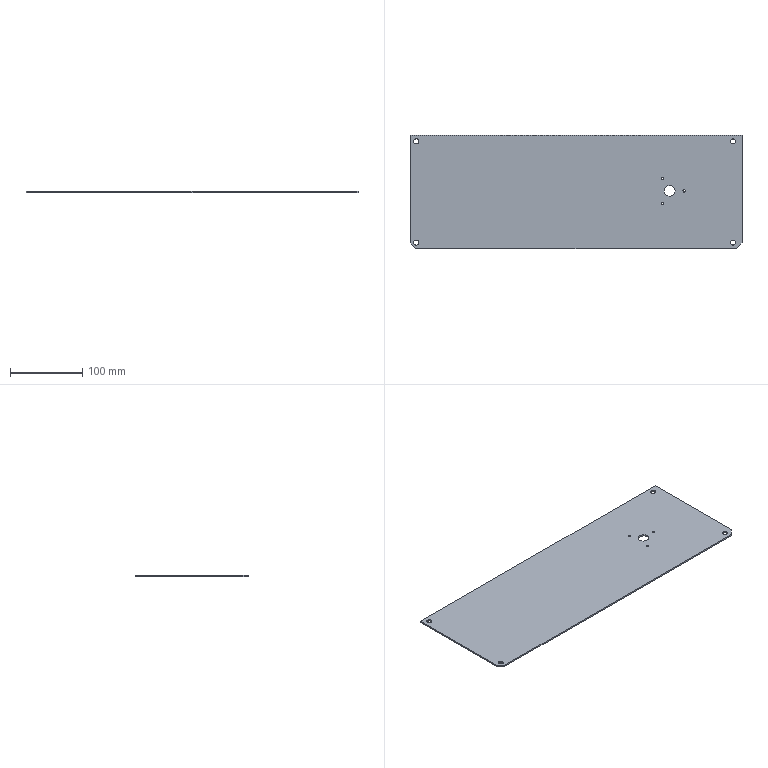Part | STEP file | Control Box Top Cover | 1 solid | 24 faces | box 459 x 157 x 2 mm | volume 143288 mm3 | cylinder 16 | plane 8 | commonest cylinder face diameters 7 x8 3.2 x6 15 x2
STEP:
#1=CARTESIAN_POINT('',(127.31,-1059.,2.));
#2=VERTEX_POINT('',#1);
#3=CARTESIAN_POINT('',(134.31,-1059.,2.));
#4=VERTEX_POINT('',#3);
#5=CARTESIAN_POINT('',(130.81,-1059.,2.));
#6=DIRECTION('',(0.,0.,1.));
#7=DIRECTION('',(-1.,0.,0.));
#8=AXIS2_PLACEMENT_3D('',#5,#6,#7);
#9=CIRCLE('',#8,3.5);
#10=EDGE_CURVE('',#2,#4,#9,.T.);
#11=ORIENTED_EDGE('',*,*,#10,.T.);
#12=CARTESIAN_POINT('',(134.31,-1059.,0.));
#13=VERTEX_POINT('',#12);
#14=CARTESIAN_POINT('',(134.31,-1059.,2.));
#15=DIRECTION('',(0.,0.,-1.));
#16=VECTOR('',#15,1000.);
#17=LINE('',#14,#16);
#18=EDGE_CURVE('',#4,#13,#17,.T.);
#19=ORIENTED_EDGE('',*,*,#18,.T.);
#20=CARTESIAN_POINT('',(127.31,-1059.,0.));
#21=VERTEX_POINT('',#20);
#22=CARTESIAN_POINT('',(130.81,-1059.,0.));
#23=DIRECTION('',(0.,0.,1.));
#24=DIRECTION('',(-1.,0.,0.));
#25=AXIS2_PLACEMENT_3D('',#22,#23,#24);
#26=CIRCLE('',#25,3.5);
#27=EDGE_CURVE('',#21,#13,#26,.T.);
#28=ORIENTED_EDGE('',*,*,#27,.F.);
#29=CARTESIAN_POINT('',(127.31,-1059.,2.));
#30=DIRECTION('',(0.,0.,-1.));
#31=VECTOR('',#30,1000.);
#32=LINE('',#29,#31);
#33=EDGE_CURVE('',#2,#21,#32,.T.);
#34=ORIENTED_EDGE('',*,*,#33,.F.);
#35=EDGE_LOOP('',(#11,#19,#28,#34));
#36=FACE_OUTER_BOUND('',#35,.T.);
#37=CARTESIAN_POINT('',(130.81,-1059.,2.));
#38=DIRECTION('',(0.,0.,-1.));
#39=DIRECTION('',(-1.,0.,0.));
#40=AXIS2_PLACEMENT_3D('',#37,#38,#39);
#41=CYLINDRICAL_SURFACE('',#40,3.5);
#42=ADVANCED_FACE('',(#36),#41,.F.);
#43=CARTESIAN_POINT('',(-310.69,-1199.,2.));
#44=VERTEX_POINT('',#43);
#45=CARTESIAN_POINT('',(-303.69,-1199.,2.));
#46=VERTEX_POINT('',#45);
#47=CARTESIAN_POINT('',(-307.19,-1199.,2.));
#48=DIRECTION('',(0.,0.,1.));
#49=DIRECTION('',(-1.,0.,0.));
#50=AXIS2_PLACEMENT_3D('',#47,#48,#49);
#51=CIRCLE('',#50,3.5);
#52=EDGE_CURVE('',#44,#46,#51,.T.);
#53=ORIENTED_EDGE('',*,*,#52,.T.);
#54=CARTESIAN_POINT('',(-303.69,-1199.,0.));
#55=VERTEX_POINT('',#54);
#56=CARTESIAN_POINT('',(-303.69,-1199.,2.));
#57=DIRECTION('',(0.,0.,-1.));
#58=VECTOR('',#57,1000.);
#59=LINE('',#56,#58);
#60=EDGE_CURVE('',#46,#55,#59,.T.);
#61=ORIENTED_EDGE('',*,*,#60,.T.);
#62=CARTESIAN_POINT('',(-310.69,-1199.,0.));
#63=VERTEX_POINT('',#62);
#64=CARTESIAN_POINT('',(-307.19,-1199.,0.));
#65=DIRECTION('',(0.,0.,1.));
#66=DIRECTION('',(-1.,0.,0.));
#67=AXIS2_PLACEMENT_3D('',#64,#65,#66);
#68=CIRCLE('',#67,3.5);
#69=EDGE_CURVE('',#63,#55,#68,.T.);
#70=ORIENTED_EDGE('',*,*,#69,.F.);
#71=CARTESIAN_POINT('',(-310.69,-1199.,2.));
#72=DIRECTION('',(0.,0.,-1.));
#73=VECTOR('',#72,1000.);
#74=LINE('',#71,#73);
#75=EDGE_CURVE('',#44,#63,#74,.T.);
#76=ORIENTED_EDGE('',*,*,#75,.F.);
#77=EDGE_LOOP('',(#53,#61,#70,#76));
#78=FACE_OUTER_BOUND('',#77,.T.);
#79=CARTESIAN_POINT('',(-307.19,-1199.,2.));
#80=DIRECTION('',(0.,0.,-1.));
#81=DIRECTION('',(-1.,0.,0.));
#82=AXIS2_PLACEMENT_3D('',#79,#80,#81);
#83=CYLINDRICAL_SURFACE('',#82,3.5);
#84=ADVANCED_FACE('',(#78),#83,.F.);
#85=CARTESIAN_POINT('',(-310.69,-1059.,2.));
#86=VERTEX_POINT('',#85);
#87=CARTESIAN_POINT('',(-303.69,-1059.,2.));
#88=VERTEX_POINT('',#87);
#89=CARTESIAN_POINT('',(-307.19,-1059.,2.));
#90=DIRECTION('',(0.,0.,1.));
#91=DIRECTION('',(-1.,0.,0.));
#92=AXIS2_PLACEMENT_3D('',#89,#90,#91);
#93=CIRCLE('',#92,3.5);
#94=EDGE_CURVE('',#86,#88,#93,.T.);
#95=ORIENTED_EDGE('',*,*,#94,.T.);
#96=CARTESIAN_POINT('',(-303.69,-1059.,0.));
#97=VERTEX_POINT('',#96);
#98=CARTESIAN_POINT('',(-303.69,-1059.,2.));
#99=DIRECTION('',(0.,0.,-1.));
#100=VECTOR('',#99,1000.);
#101=LINE('',#98,#100);
#102=EDGE_CURVE('',#88,#97,#101,.T.);
#103=ORIENTED_EDGE('',*,*,#102,.T.);
#104=CARTESIAN_POINT('',(-310.69,-1059.,0.));
#105=VERTEX_POINT('',#104);
#106=CARTESIAN_POINT('',(-307.19,-1059.,0.));
#107=DIRECTION('',(0.,0.,1.));
#108=DIRECTION('',(-1.,0.,0.));
#109=AXIS2_PLACEMENT_3D('',#106,#107,#108);
#110=CIRCLE('',#109,3.5);
#111=EDGE_CURVE('',#105,#97,#110,.T.);
#112=ORIENTED_EDGE('',*,*,#111,.F.);
#113=CARTESIAN_POINT('',(-310.69,-1059.,2.));
#114=DIRECTION('',(0.,0.,-1.));
#115=VECTOR('',#114,1000.);
#116=LINE('',#113,#115);
#117=EDGE_CURVE('',#86,#105,#116,.T.);
#118=ORIENTED_EDGE('',*,*,#117,.F.);
#119=EDGE_LOOP('',(#95,#103,#112,#118));
#120=FACE_OUTER_BOUND('',#119,.T.);
#121=CARTESIAN_POINT('',(-307.19,-1059.,2.));
#122=DIRECTION('',(0.,0.,-1.));
#123=DIRECTION('',(-1.,0.,0.));
#124=AXIS2_PLACEMENT_3D('',#121,#122,#123);
#125=CYLINDRICAL_SURFACE('',#124,3.5);
#126=ADVANCED_FACE('',(#120),#125,.F.);
#127=CARTESIAN_POINT('',(127.31,-1199.,2.));
#128=VERTEX_POINT('',#127);
#129=CARTESIAN_POINT('',(134.31,-1199.,2.));
#130=VERTEX_POINT('',#129);
#131=CARTESIAN_POINT('',(130.81,-1199.,2.));
#132=DIRECTION('',(0.,0.,1.));
#133=DIRECTION('',(-1.,0.,0.));
#134=AXIS2_PLACEMENT_3D('',#131,#132,#133);
#135=CIRCLE('',#134,3.5);
#136=EDGE_CURVE('',#128,#130,#135,.T.);
#137=ORIENTED_EDGE('',*,*,#136,.T.);
#138=CARTESIAN_POINT('',(134.31,-1199.,0.));
#139=VERTEX_POINT('',#138);
#140=CARTESIAN_POINT('',(134.31,-1199.,2.));
#141=DIRECTION('',(0.,0.,-1.));
#142=VECTOR('',#141,1000.);
#143=LINE('',#140,#142);
#144=EDGE_CURVE('',#130,#139,#143,.T.);
#145=ORIENTED_EDGE('',*,*,#144,.T.);
#146=CARTESIAN_POINT('',(127.31,-1199.,0.));
#147=VERTEX_POINT('',#146);
#148=CARTESIAN_POINT('',(130.81,-1199.,0.));
#149=DIRECTION('',(0.,0.,1.));
#150=DIRECTION('',(-1.,0.,0.));
#151=AXIS2_PLACEMENT_3D('',#148,#149,#150);
#152=CIRCLE('',#151,3.5);
#153=EDGE_CURVE('',#147,#139,#152,.T.);
#154=ORIENTED_EDGE('',*,*,#153,.F.);
#155=CARTESIAN_POINT('',(127.31,-1199.,2.));
#156=DIRECTION('',(0.,0.,-1.));
#157=VECTOR('',#156,1000.);
#158=LINE('',#155,#157);
#159=EDGE_CURVE('',#128,#147,#158,.T.);
#160=ORIENTED_EDGE('',*,*,#159,.F.);
#161=EDGE_LOOP('',(#137,#145,#154,#160));
#162=FACE_OUTER_BOUND('',#161,.T.);
#163=CARTESIAN_POINT('',(130.81,-1199.,2.));
#164=DIRECTION('',(0.,0.,-1.));
#165=DIRECTION('',(-1.,0.,0.));
#166=AXIS2_PLACEMENT_3D('',#163,#164,#165);
#167=CYLINDRICAL_SURFACE('',#166,3.5);
#168=ADVANCED_FACE('',(#162),#167,.F.);
#169=CARTESIAN_POINT('',(35.81,-1127.5,0.));
#170=VERTEX_POINT('',#169);
#171=CARTESIAN_POINT('',(50.81,-1127.5,0.));
#172=VERTEX_POINT('',#171);
#173=CARTESIAN_POINT('',(43.31,-1127.5,0.));
#174=DIRECTION('',(0.,0.,1.));
#175=DIRECTION('',(1.,0.,0.));
#176=AXIS2_PLACEMENT_3D('',#173,#174,#175);
#177=CIRCLE('',#176,7.5);
#178=EDGE_CURVE('',#170,#172,#177,.T.);
#179=ORIENTED_EDGE('',*,*,#178,.F.);
#180=CARTESIAN_POINT('',(35.81,-1127.5,2.));
#181=VERTEX_POINT('',#180);
#182=CARTESIAN_POINT('',(35.81,-1127.5,-8.));
#183=DIRECTION('',(0.,0.,1.));
#184=VECTOR('',#183,1000.);
#185=LINE('',#182,#184);
#186=EDGE_CURVE('',#170,#181,#185,.T.);
#187=ORIENTED_EDGE('',*,*,#186,.T.);
#188=CARTESIAN_POINT('',(50.81,-1127.5,2.));
#189=VERTEX_POINT('',#188);
#190=CARTESIAN_POINT('',(43.31,-1127.5,2.));
#191=DIRECTION('',(0.,0.,1.));
#192=DIRECTION('',(1.,0.,0.));
#193=AXIS2_PLACEMENT_3D('',#190,#191,#192);
#194=CIRCLE('',#193,7.5);
#195=EDGE_CURVE('',#181,#189,#194,.T.);
#196=ORIENTED_EDGE('',*,*,#195,.T.);
#197=CARTESIAN_POINT('',(50.81,-1127.5,-8.));
#198=DIRECTION('',(0.,0.,1.));
#199=VECTOR('',#198,1000.);
#200=LINE('',#197,#199);
#201=EDGE_CURVE('',#172,#189,#200,.T.);
#202=ORIENTED_EDGE('',*,*,#201,.F.);
#203=EDGE_LOOP('',(#179,#187,#196,#202));
#204=FACE_OUTER_BOUND('',#203,.T.);
#205=CARTESIAN_POINT('',(43.31,-1127.5,-8.));
#206=DIRECTION('',(0.,0.,1.));
#207=DIRECTION('',(1.,0.,0.));
#208=AXIS2_PLACEMENT_3D('',#205,#206,#207);
#209=CYLINDRICAL_SURFACE('',#208,7.5);
#210=ADVANCED_FACE('',(#204),#209,.F.);
#211=CARTESIAN_POINT('',(61.71,-1127.5,0.));
#212=VERTEX_POINT('',#211);
#213=CARTESIAN_POINT('',(64.91,-1127.5,0.));
#214=VERTEX_POINT('',#213);
#215=CARTESIAN_POINT('',(63.31,-1127.5,0.));
#216=DIRECTION('',(0.,0.,1.));
#217=DIRECTION('',(1.,0.,0.));
#218=AXIS2_PLACEMENT_3D('',#215,#216,#217);
#219=CIRCLE('',#218,1.6);
#220=EDGE_CURVE('',#212,#214,#219,.T.);
#221=ORIENTED_EDGE('',*,*,#220,.F.);
#222=CARTESIAN_POINT('',(61.71,-1127.5,2.));
#223=VERTEX_POINT('',#222);
#224=CARTESIAN_POINT('',(61.71,-1127.5,-8.));
#225=DIRECTION('',(0.,0.,1.));
#226=VECTOR('',#225,1000.);
#227=LINE('',#224,#226);
#228=EDGE_CURVE('',#212,#223,#227,.T.);
#229=ORIENTED_EDGE('',*,*,#228,.T.);
#230=CARTESIAN_POINT('',(64.91,-1127.5,2.));
#231=VERTEX_POINT('',#230);
#232=CARTESIAN_POINT('',(63.31,-1127.5,2.));
#233=DIRECTION('',(0.,0.,1.));
#234=DIRECTION('',(1.,0.,0.));
#235=AXIS2_PLACEMENT_3D('',#232,#233,#234);
#236=CIRCLE('',#235,1.6);
#237=EDGE_CURVE('',#223,#231,#236,.T.);
#238=ORIENTED_EDGE('',*,*,#237,.T.);
#239=CARTESIAN_POINT('',(64.91,-1127.5,-8.));
#240=DIRECTION('',(0.,0.,1.));
#241=VECTOR('',#240,1000.);
#242=LINE('',#239,#241);
#243=EDGE_CURVE('',#214,#231,#242,.T.);
#244=ORIENTED_EDGE('',*,*,#243,.F.);
#245=EDGE_LOOP('',(#221,#229,#238,#244));
#246=FACE_OUTER_BOUND('',#245,.T.);
#247=CARTESIAN_POINT('',(63.31,-1127.5,-8.));
#248=DIRECTION('',(0.,0.,1.));
#249=DIRECTION('',(1.,0.,0.));
#250=AXIS2_PLACEMENT_3D('',#247,#248,#249);
#251=CYLINDRICAL_SURFACE('',#250,1.6);
#252=ADVANCED_FACE('',(#246),#251,.F.);
#253=CARTESIAN_POINT('',(31.71,-1144.821,0.));
#254=VERTEX_POINT('',#253);
#255=CARTESIAN_POINT('',(34.91,-1144.821,0.));
#256=VERTEX_POINT('',#255);
#257=CARTESIAN_POINT('',(33.31,-1144.821,0.));
#258=DIRECTION('',(0.,0.,1.));
#259=DIRECTION('',(1.,0.,0.));
#260=AXIS2_PLACEMENT_3D('',#257,#258,#259);
#261=CIRCLE('',#260,1.6);
#262=EDGE_CURVE('',#254,#256,#261,.T.);
#263=ORIENTED_EDGE('',*,*,#262,.F.);
#264=CARTESIAN_POINT('',(31.71,-1144.821,2.));
#265=VERTEX_POINT('',#264);
#266=CARTESIAN_POINT('',(31.71,-1144.821,-8.));
#267=DIRECTION('',(0.,0.,1.));
#268=VECTOR('',#267,1000.);
#269=LINE('',#266,#268);
#270=EDGE_CURVE('',#254,#265,#269,.T.);
#271=ORIENTED_EDGE('',*,*,#270,.T.);
#272=CARTESIAN_POINT('',(34.91,-1144.821,2.));
#273=VERTEX_POINT('',#272);
#274=CARTESIAN_POINT('',(33.31,-1144.821,2.));
#275=DIRECTION('',(0.,0.,1.));
#276=DIRECTION('',(1.,0.,0.));
#277=AXIS2_PLACEMENT_3D('',#274,#275,#276);
#278=CIRCLE('',#277,1.6);
#279=EDGE_CURVE('',#265,#273,#278,.T.);
#280=ORIENTED_EDGE('',*,*,#279,.T.);
#281=CARTESIAN_POINT('',(34.91,-1144.821,-8.));
#282=DIRECTION('',(0.,0.,1.));
#283=VECTOR('',#282,1000.);
#284=LINE('',#281,#283);
#285=EDGE_CURVE('',#256,#273,#284,.T.);
#286=ORIENTED_EDGE('',*,*,#285,.F.);
#287=EDGE_LOOP('',(#263,#271,#280,#286));
#288=FACE_OUTER_BOUND('',#287,.T.);
#289=CARTESIAN_POINT('',(33.31,-1144.821,-8.));
#290=DIRECTION('',(0.,0.,1.));
#291=DIRECTION('',(1.,0.,0.));
#292=AXIS2_PLACEMENT_3D('',#289,#290,#291);
#293=CYLINDRICAL_SURFACE('',#292,1.6);
#294=ADVANCED_FACE('',(#288),#293,.F.);
#295=CARTESIAN_POINT('',(31.71,-1110.179,0.));
#296=VERTEX_POINT('',#295);
#297=CARTESIAN_POINT('',(34.91,-1110.179,0.));
#298=VERTEX_POINT('',#297);
#299=CARTESIAN_POINT('',(33.31,-1110.179,0.));
#300=DIRECTION('',(0.,0.,1.));
#301=DIRECTION('',(1.,0.,0.));
#302=AXIS2_PLACEMENT_3D('',#299,#300,#301);
#303=CIRCLE('',#302,1.6);
#304=EDGE_CURVE('',#296,#298,#303,.T.);
#305=ORIENTED_EDGE('',*,*,#304,.F.);
#306=CARTESIAN_POINT('',(31.71,-1110.179,2.));
#307=VERTEX_POINT('',#306);
#308=CARTESIAN_POINT('',(31.71,-1110.179,-8.));
#309=DIRECTION('',(0.,0.,1.));
#310=VECTOR('',#309,1000.);
#311=LINE('',#308,#310);
#312=EDGE_CURVE('',#296,#307,#311,.T.);
#313=ORIENTED_EDGE('',*,*,#312,.T.);
#314=CARTESIAN_POINT('',(34.91,-1110.179,2.));
#315=VERTEX_POINT('',#314);
#316=CARTESIAN_POINT('',(33.31,-1110.179,2.));
#317=DIRECTION('',(0.,0.,1.));
#318=DIRECTION('',(1.,0.,0.));
#319=AXIS2_PLACEMENT_3D('',#316,#317,#318);
#320=CIRCLE('',#319,1.6);
#321=EDGE_CURVE('',#307,#315,#320,.T.);
#322=ORIENTED_EDGE('',*,*,#321,.T.);
#323=CARTESIAN_POINT('',(34.91,-1110.179,-8.));
#324=DIRECTION('',(0.,0.,1.));
#325=VECTOR('',#324,1000.);
#326=LINE('',#323,#325);
#327=EDGE_CURVE('',#298,#315,#326,.T.);
#328=ORIENTED_EDGE('',*,*,#327,.F.);
#329=EDGE_LOOP('',(#305,#313,#322,#328));
#330=FACE_OUTER_BOUND('',#329,.T.);
#331=CARTESIAN_POINT('',(33.31,-1110.179,-8.));
#332=DIRECTION('',(0.,0.,1.));
#333=DIRECTION('',(1.,0.,0.));
#334=AXIS2_PLACEMENT_3D('',#331,#332,#333);
#335=CYLINDRICAL_SURFACE('',#334,1.6);
#336=ADVANCED_FACE('',(#330),#335,.F.);
#337=ORIENTED_EDGE('',*,*,#10,.F.);
#338=CARTESIAN_POINT('',(130.81,-1059.,2.));
#339=DIRECTION('',(0.,0.,1.));
#340=DIRECTION('',(-1.,0.,0.));
#341=AXIS2_PLACEMENT_3D('',#338,#339,#340);
#342=CIRCLE('',#341,3.5);
#343=EDGE_CURVE('',#4,#2,#342,.T.);
#344=ORIENTED_EDGE('',*,*,#343,.F.);
#345=EDGE_LOOP('',(#337,#344));
#346=FACE_BOUND('',#345,.T.);
#347=ORIENTED_EDGE('',*,*,#52,.F.);
#348=CARTESIAN_POINT('',(-307.19,-1199.,2.));
#349=DIRECTION('',(0.,0.,1.));
#350=DIRECTION('',(-1.,0.,0.));
#351=AXIS2_PLACEMENT_3D('',#348,#349,#350);
#352=CIRCLE('',#351,3.5);
#353=EDGE_CURVE('',#46,#44,#352,.T.);
#354=ORIENTED_EDGE('',*,*,#353,.F.);
#355=EDGE_LOOP('',(#347,#354));
#356=FACE_BOUND('',#355,.T.);
#357=CARTESIAN_POINT('',(143.31,-1199.5,2.));
#358=VERTEX_POINT('',#357);
#359=CARTESIAN_POINT('',(135.31,-1207.5,2.));
#360=VERTEX_POINT('',#359);
#361=CARTESIAN_POINT('',(143.31,-1199.5,2.));
#362=DIRECTION('',(-0.7071,-0.7071,0.));
#363=VECTOR('',#362,1000.);
#364=LINE('',#361,#363);
#365=EDGE_CURVE('',#358,#360,#364,.T.);
#366=ORIENTED_EDGE('',*,*,#365,.F.);
#367=CARTESIAN_POINT('',(143.31,-1050.5,2.));
#368=VERTEX_POINT('',#367);
#369=CARTESIAN_POINT('',(143.31,0.,2.));
#370=DIRECTION('',(0.,-1.,0.));
#371=VECTOR('',#370,1000.);
#372=LINE('',#369,#371);
#373=EDGE_CURVE('',#368,#358,#372,.T.);
#374=ORIENTED_EDGE('',*,*,#373,.F.);
#375=CARTESIAN_POINT('',(-315.69,-1050.5,2.));
#376=VERTEX_POINT('',#375);
#377=CARTESIAN_POINT('',(0.,-1050.5,2.));
#378=DIRECTION('',(1.,0.,0.));
#379=VECTOR('',#378,1000.);
#380=LINE('',#377,#379);
#381=EDGE_CURVE('',#376,#368,#380,.T.);
#382=ORIENTED_EDGE('',*,*,#381,.F.);
#383=CARTESIAN_POINT('',(-315.69,-1199.5,2.));
#384=VERTEX_POINT('',#383);
#385=CARTESIAN_POINT('',(-315.69,0.,2.));
#386=DIRECTION('',(0.,1.,0.));
#387=VECTOR('',#386,1000.);
#388=LINE('',#385,#387);
#389=EDGE_CURVE('',#384,#376,#388,.T.);
#390=ORIENTED_EDGE('',*,*,#389,.F.);
#391=CARTESIAN_POINT('',(-307.69,-1207.5,2.));
#392=VERTEX_POINT('',#391);
#393=CARTESIAN_POINT('',(-307.69,-1207.5,2.));
#394=DIRECTION('',(-0.7071,0.7071,0.));
#395=VECTOR('',#394,1000.);
#396=LINE('',#393,#395);
#397=EDGE_CURVE('',#392,#384,#396,.T.);
#398=ORIENTED_EDGE('',*,*,#397,.F.);
#399=CARTESIAN_POINT('',(0.,-1207.5,2.));
#400=DIRECTION('',(-1.,0.,0.));
#401=VECTOR('',#400,1000.);
#402=LINE('',#399,#401);
#403=EDGE_CURVE('',#360,#392,#402,.T.);
#404=ORIENTED_EDGE('',*,*,#403,.F.);
#405=EDGE_LOOP('',(#366,#374,#382,#390,#398,#404));
#406=FACE_OUTER_BOUND('',#405,.T.);
#407=ORIENTED_EDGE('',*,*,#94,.F.);
#408=CARTESIAN_POINT('',(-307.19,-1059.,2.));
#409=DIRECTION('',(0.,0.,1.));
#410=DIRECTION('',(-1.,0.,0.));
#411=AXIS2_PLACEMENT_3D('',#408,#409,#410);
#412=CIRCLE('',#411,3.5);
#413=EDGE_CURVE('',#88,#86,#412,.T.);
#414=ORIENTED_EDGE('',*,*,#413,.F.);
#415=EDGE_LOOP('',(#407,#414));
#416=FACE_BOUND('',#415,.T.);
#417=ORIENTED_EDGE('',*,*,#136,.F.);
#418=CARTESIAN_POINT('',(130.81,-1199.,2.));
#419=DIRECTION('',(0.,0.,1.));
#420=DIRECTION('',(-1.,0.,0.));
#421=AXIS2_PLACEMENT_3D('',#418,#419,#420);
#422=CIRCLE('',#421,3.5);
#423=EDGE_CURVE('',#130,#128,#422,.T.);
#424=ORIENTED_EDGE('',*,*,#423,.F.);
#425=EDGE_LOOP('',(#417,#424));
#426=FACE_BOUND('',#425,.T.);
#427=CARTESIAN_POINT('',(43.31,-1127.5,2.));
#428=DIRECTION('',(0.,0.,1.));
#429=DIRECTION('',(1.,0.,0.));
#430=AXIS2_PLACEMENT_3D('',#427,#428,#429);
#431=CIRCLE('',#430,7.5);
#432=EDGE_CURVE('',#189,#181,#431,.T.);
#433=ORIENTED_EDGE('',*,*,#432,.F.);
#434=ORIENTED_EDGE('',*,*,#195,.F.);
#435=EDGE_LOOP('',(#433,#434));
#436=FACE_BOUND('',#435,.T.);
#437=CARTESIAN_POINT('',(63.31,-1127.5,2.));
#438=DIRECTION('',(0.,0.,1.));
#439=DIRECTION('',(1.,0.,0.));
#440=AXIS2_PLACEMENT_3D('',#437,#438,#439);
#441=CIRCLE('',#440,1.6);
#442=EDGE_CURVE('',#231,#223,#441,.T.);
#443=ORIENTED_EDGE('',*,*,#442,.F.);
#444=ORIENTED_EDGE('',*,*,#237,.F.);
#445=EDGE_LOOP('',(#443,#444));
#446=FACE_BOUND('',#445,.T.);
#447=CARTESIAN_POINT('',(33.31,-1144.821,2.));
#448=DIRECTION('',(0.,0.,1.));
#449=DIRECTION('',(1.,0.,0.));
#450=AXIS2_PLACEMENT_3D('',#447,#448,#449);
#451=CIRCLE('',#450,1.6);
#452=EDGE_CURVE('',#273,#265,#451,.T.);
#453=ORIENTED_EDGE('',*,*,#452,.F.);
#454=ORIENTED_EDGE('',*,*,#279,.F.);
#455=EDGE_LOOP('',(#453,#454));
#456=FACE_BOUND('',#455,.T.);
#457=CARTESIAN_POINT('',(33.31,-1110.179,2.));
#458=DIRECTION('',(0.,0.,1.));
#459=DIRECTION('',(1.,0.,0.));
#460=AXIS2_PLACEMENT_3D('',#457,#458,#459);
#461=CIRCLE('',#460,1.6);
#462=EDGE_CURVE('',#315,#307,#461,.T.);
#463=ORIENTED_EDGE('',*,*,#462,.F.);
#464=ORIENTED_EDGE('',*,*,#321,.F.);
#465=EDGE_LOOP('',(#463,#464));
#466=FACE_BOUND('',#465,.T.);
#467=CARTESIAN_POINT('',(0.,0.,2.));
#468=DIRECTION('',(0.,0.,-1.));
#469=DIRECTION('',(-1.,0.,0.));
#470=AXIS2_PLACEMENT_3D('',#467,#468,#469);
#471=PLANE('',#470);
#472=ADVANCED_FACE('',(#346,#356,#406,#416,#426,#436,#446,#456,#466),#471,.F.);
#473=ORIENTED_EDGE('',*,*,#18,.F.);
#474=ORIENTED_EDGE('',*,*,#343,.T.);
#475=ORIENTED_EDGE('',*,*,#33,.T.);
#476=CARTESIAN_POINT('',(130.81,-1059.,0.));
#477=DIRECTION('',(0.,0.,1.));
#478=DIRECTION('',(-1.,0.,0.));
#479=AXIS2_PLACEMENT_3D('',#476,#477,#478);
#480=CIRCLE('',#479,3.5);
#481=EDGE_CURVE('',#13,#21,#480,.T.);
#482=ORIENTED_EDGE('',*,*,#481,.F.);
#483=EDGE_LOOP('',(#473,#474,#475,#482));
#484=FACE_OUTER_BOUND('',#483,.T.);
#485=CARTESIAN_POINT('',(130.81,-1059.,2.));
#486=DIRECTION('',(0.,0.,-1.));
#487=DIRECTION('',(-1.,0.,0.));
#488=AXIS2_PLACEMENT_3D('',#485,#486,#487);
#489=CYLINDRICAL_SURFACE('',#488,3.5);
#490=ADVANCED_FACE('',(#484),#489,.F.);
#491=ORIENTED_EDGE('',*,*,#60,.F.);
#492=ORIENTED_EDGE('',*,*,#353,.T.);
#493=ORIENTED_EDGE('',*,*,#75,.T.);
#494=CARTESIAN_POINT('',(-307.19,-1199.,0.));
#495=DIRECTION('',(0.,0.,1.));
#496=DIRECTION('',(-1.,0.,0.));
#497=AXIS2_PLACEMENT_3D('',#494,#495,#496);
#498=CIRCLE('',#497,3.5);
#499=EDGE_CURVE('',#55,#63,#498,.T.);
#500=ORIENTED_EDGE('',*,*,#499,.F.);
#501=EDGE_LOOP('',(#491,#492,#493,#500));
#502=FACE_OUTER_BOUND('',#501,.T.);
#503=CARTESIAN_POINT('',(-307.19,-1199.,2.));
#504=DIRECTION('',(0.,0.,-1.));
#505=DIRECTION('',(-1.,0.,0.));
#506=AXIS2_PLACEMENT_3D('',#503,#504,#505);
#507=CYLINDRICAL_SURFACE('',#506,3.5);
#508=ADVANCED_FACE('',(#502),#507,.F.);
#509=CARTESIAN_POINT('',(135.31,-1207.5,0.));
#510=VERTEX_POINT('',#509);
#511=CARTESIAN_POINT('',(135.31,-1207.5,2.));
#512=DIRECTION('',(0.,0.,-1.));
#513=VECTOR('',#512,1000.);
#514=LINE('',#511,#513);
#515=EDGE_CURVE('',#360,#510,#514,.T.);
#516=ORIENTED_EDGE('',*,*,#515,.F.);
#517=ORIENTED_EDGE('',*,*,#403,.T.);
#518=CARTESIAN_POINT('',(-307.69,-1207.5,0.));
#519=VERTEX_POINT('',#518);
#520=CARTESIAN_POINT('',(-307.69,-1207.5,2.));
#521=DIRECTION('',(0.,0.,1.));
#522=VECTOR('',#521,1000.);
#523=LINE('',#520,#522);
#524=EDGE_CURVE('',#519,#392,#523,.T.);
#525=ORIENTED_EDGE('',*,*,#524,.F.);
#526=CARTESIAN_POINT('',(-315.69,-1207.5,0.));
#527=DIRECTION('',(-1.,0.,0.));
#528=VECTOR('',#527,1000.);
#529=LINE('',#526,#528);
#530=EDGE_CURVE('',#510,#519,#529,.T.);
#531=ORIENTED_EDGE('',*,*,#530,.F.);
#532=EDGE_LOOP('',(#516,#517,#525,#531));
#533=FACE_OUTER_BOUND('',#532,.T.);
#534=CARTESIAN_POINT('',(-315.69,-1207.5,2.));
#535=DIRECTION('',(0.,1.,0.));
#536=DIRECTION('',(-1.,0.,0.));
#537=AXIS2_PLACEMENT_3D('',#534,#535,#536);
#538=PLANE('',#537);
#539=ADVANCED_FACE('',(#533),#538,.F.);
#540=ORIENTED_EDGE('',*,*,#515,.T.);
#541=CARTESIAN_POINT('',(143.31,-1199.5,0.));
#542=VERTEX_POINT('',#541);
#543=CARTESIAN_POINT('',(143.31,-1199.5,0.));
#544=DIRECTION('',(-0.7071,-0.7071,0.));
#545=VECTOR('',#544,1000.);
#546=LINE('',#543,#545);
#547=EDGE_CURVE('',#542,#510,#546,.T.);
#548=ORIENTED_EDGE('',*,*,#547,.F.);
#549=CARTESIAN_POINT('',(143.31,-1199.5,2.));
#550=DIRECTION('',(0.,0.,-1.));
#551=VECTOR('',#550,1000.);
#552=LINE('',#549,#551);
#553=EDGE_CURVE('',#358,#542,#552,.T.);
#554=ORIENTED_EDGE('',*,*,#553,.F.);
#555=ORIENTED_EDGE('',*,*,#365,.T.);
#556=EDGE_LOOP('',(#540,#548,#554,#555));
#557=FACE_OUTER_BOUND('',#556,.T.);
#558=CARTESIAN_POINT('',(143.31,-1199.5,2.));
#559=DIRECTION('',(-0.7071,0.7071,0.));
#560=DIRECTION('',(-0.7071,-0.7071,0.));
#561=AXIS2_PLACEMENT_3D('',#558,#559,#560);
#562=PLANE('',#561);
#563=ADVANCED_FACE('',(#557),#562,.F.);
#564=ORIENTED_EDGE('',*,*,#553,.T.);
#565=CARTESIAN_POINT('',(143.31,-1050.5,0.));
#566=VERTEX_POINT('',#565);
#567=CARTESIAN_POINT('',(143.31,-1050.5,0.));
#568=DIRECTION('',(0.,-1.,0.));
#569=VECTOR('',#568,1000.);
#570=LINE('',#567,#569);
#571=EDGE_CURVE('',#566,#542,#570,.T.);
#572=ORIENTED_EDGE('',*,*,#571,.F.);
#573=CARTESIAN_POINT('',(143.31,-1050.5,2.));
#574=DIRECTION('',(0.,0.,-1.));
#575=VECTOR('',#574,1000.);
#576=LINE('',#573,#575);
#577=EDGE_CURVE('',#368,#566,#576,.T.);
#578=ORIENTED_EDGE('',*,*,#577,.F.);
#579=ORIENTED_EDGE('',*,*,#373,.T.);
#580=EDGE_LOOP('',(#564,#572,#578,#579));
#581=FACE_OUTER_BOUND('',#580,.T.);
#582=CARTESIAN_POINT('',(143.31,-1050.5,2.));
#583=DIRECTION('',(-1.,0.,0.));
#584=DIRECTION('',(0.,0.,1.));
#585=AXIS2_PLACEMENT_3D('',#582,#583,#584);
#586=PLANE('',#585);
#587=ADVANCED_FACE('',(#581),#586,.F.);
#588=CARTESIAN_POINT('',(-315.69,-1050.5,0.));
#589=VERTEX_POINT('',#588);
#590=CARTESIAN_POINT('',(-315.69,-1050.5,2.));
#591=DIRECTION('',(0.,0.,-1.));
#592=VECTOR('',#591,1000.);
#593=LINE('',#590,#592);
#594=EDGE_CURVE('',#376,#589,#593,.T.);
#595=ORIENTED_EDGE('',*,*,#594,.F.);
#596=ORIENTED_EDGE('',*,*,#381,.T.);
#597=ORIENTED_EDGE('',*,*,#577,.T.);
#598=CARTESIAN_POINT('',(-315.69,-1050.5,0.));
#599=DIRECTION('',(1.,0.,0.));
#600=VECTOR('',#599,1000.);
#601=LINE('',#598,#600);
#602=EDGE_CURVE('',#589,#566,#601,.T.);
#603=ORIENTED_EDGE('',*,*,#602,.F.);
#604=EDGE_LOOP('',(#595,#596,#597,#603));
#605=FACE_OUTER_BOUND('',#604,.T.);
#606=CARTESIAN_POINT('',(-315.69,-1050.5,2.));
#607=DIRECTION('',(0.,-1.,0.));
#608=DIRECTION('',(1.,0.,0.));
#609=AXIS2_PLACEMENT_3D('',#606,#607,#608);
#610=PLANE('',#609);
#611=ADVANCED_FACE('',(#605),#610,.F.);
#612=CARTESIAN_POINT('',(-315.69,-1199.5,0.));
#613=VERTEX_POINT('',#612);
#614=CARTESIAN_POINT('',(-315.69,-1199.5,2.));
#615=DIRECTION('',(0.,0.,-1.));
#616=VECTOR('',#615,1000.);
#617=LINE('',#614,#616);
#618=EDGE_CURVE('',#384,#613,#617,.T.);
#619=ORIENTED_EDGE('',*,*,#618,.F.);
#620=ORIENTED_EDGE('',*,*,#389,.T.);
#621=ORIENTED_EDGE('',*,*,#594,.T.);
#622=CARTESIAN_POINT('',(-315.69,-1050.5,0.));
#623=DIRECTION('',(0.,1.,0.));
#624=VECTOR('',#623,1000.);
#625=LINE('',#622,#624);
#626=EDGE_CURVE('',#613,#589,#625,.T.);
#627=ORIENTED_EDGE('',*,*,#626,.F.);
#628=EDGE_LOOP('',(#619,#620,#621,#627));
#629=FACE_OUTER_BOUND('',#628,.T.);
#630=CARTESIAN_POINT('',(-315.69,-1050.5,2.));
#631=DIRECTION('',(1.,0.,0.));
#632=DIRECTION('',(0.,0.,-1.));
#633=AXIS2_PLACEMENT_3D('',#630,#631,#632);
#634=PLANE('',#633);
#635=ADVANCED_FACE('',(#629),#634,.F.);
#636=ORIENTED_EDGE('',*,*,#618,.T.);
#637=CARTESIAN_POINT('',(-307.69,-1207.5,0.));
#638=DIRECTION('',(-0.7071,0.7071,0.));
#639=VECTOR('',#638,1000.);
#640=LINE('',#637,#639);
#641=EDGE_CURVE('',#519,#613,#640,.T.);
#642=ORIENTED_EDGE('',*,*,#641,.F.);
#643=ORIENTED_EDGE('',*,*,#524,.T.);
#644=ORIENTED_EDGE('',*,*,#397,.T.);
#645=EDGE_LOOP('',(#636,#642,#643,#644));
#646=FACE_OUTER_BOUND('',#645,.T.);
#647=CARTESIAN_POINT('',(-307.69,-1207.5,2.));
#648=DIRECTION('',(0.7071,0.7071,0.));
#649=DIRECTION('',(-0.7071,0.7071,0.));
#650=AXIS2_PLACEMENT_3D('',#647,#648,#649);
#651=PLANE('',#650);
#652=ADVANCED_FACE('',(#646),#651,.F.);
#653=ORIENTED_EDGE('',*,*,#102,.F.);
#654=ORIENTED_EDGE('',*,*,#413,.T.);
#655=ORIENTED_EDGE('',*,*,#117,.T.);
#656=CARTESIAN_POINT('',(-307.19,-1059.,0.));
#657=DIRECTION('',(0.,0.,1.));
#658=DIRECTION('',(-1.,0.,0.));
#659=AXIS2_PLACEMENT_3D('',#656,#657,#658);
#660=CIRCLE('',#659,3.5);
#661=EDGE_CURVE('',#97,#105,#660,.T.);
#662=ORIENTED_EDGE('',*,*,#661,.F.);
#663=EDGE_LOOP('',(#653,#654,#655,#662));
#664=FACE_OUTER_BOUND('',#663,.T.);
#665=CARTESIAN_POINT('',(-307.19,-1059.,2.));
#666=DIRECTION('',(0.,0.,-1.));
#667=DIRECTION('',(-1.,0.,0.));
#668=AXIS2_PLACEMENT_3D('',#665,#666,#667);
#669=CYLINDRICAL_SURFACE('',#668,3.5);
#670=ADVANCED_FACE('',(#664),#669,.F.);
#671=ORIENTED_EDGE('',*,*,#144,.F.);
#672=ORIENTED_EDGE('',*,*,#423,.T.);
#673=ORIENTED_EDGE('',*,*,#159,.T.);
#674=CARTESIAN_POINT('',(130.81,-1199.,0.));
#675=DIRECTION('',(0.,0.,1.));
#676=DIRECTION('',(-1.,0.,0.));
#677=AXIS2_PLACEMENT_3D('',#674,#675,#676);
#678=CIRCLE('',#677,3.5);
#679=EDGE_CURVE('',#139,#147,#678,.T.);
#680=ORIENTED_EDGE('',*,*,#679,.F.);
#681=EDGE_LOOP('',(#671,#672,#673,#680));
#682=FACE_OUTER_BOUND('',#681,.T.);
#683=CARTESIAN_POINT('',(130.81,-1199.,2.));
#684=DIRECTION('',(0.,0.,-1.));
#685=DIRECTION('',(-1.,0.,0.));
#686=AXIS2_PLACEMENT_3D('',#683,#684,#685);
#687=CYLINDRICAL_SURFACE('',#686,3.5);
#688=ADVANCED_FACE('',(#682),#687,.F.);
#689=ORIENTED_EDGE('',*,*,#186,.F.);
#690=CARTESIAN_POINT('',(43.31,-1127.5,0.));
#691=DIRECTION('',(0.,0.,1.));
#692=DIRECTION('',(1.,0.,0.));
#693=AXIS2_PLACEMENT_3D('',#690,#691,#692);
#694=CIRCLE('',#693,7.5);
#695=EDGE_CURVE('',#172,#170,#694,.T.);
#696=ORIENTED_EDGE('',*,*,#695,.F.);
#697=ORIENTED_EDGE('',*,*,#201,.T.);
#698=ORIENTED_EDGE('',*,*,#432,.T.);
#699=EDGE_LOOP('',(#689,#696,#697,#698));
#700=FACE_OUTER_BOUND('',#699,.T.);
#701=CARTESIAN_POINT('',(43.31,-1127.5,-8.));
#702=DIRECTION('',(0.,0.,1.));
#703=DIRECTION('',(1.,0.,0.));
#704=AXIS2_PLACEMENT_3D('',#701,#702,#703);
#705=CYLINDRICAL_SURFACE('',#704,7.5);
#706=ADVANCED_FACE('',(#700),#705,.F.);
#707=ORIENTED_EDGE('',*,*,#228,.F.);
#708=CARTESIAN_POINT('',(63.31,-1127.5,0.));
#709=DIRECTION('',(0.,0.,1.));
#710=DIRECTION('',(1.,0.,0.));
#711=AXIS2_PLACEMENT_3D('',#708,#709,#710);
#712=CIRCLE('',#711,1.6);
#713=EDGE_CURVE('',#214,#212,#712,.T.);
#714=ORIENTED_EDGE('',*,*,#713,.F.);
#715=ORIENTED_EDGE('',*,*,#243,.T.);
#716=ORIENTED_EDGE('',*,*,#442,.T.);
#717=EDGE_LOOP('',(#707,#714,#715,#716));
#718=FACE_OUTER_BOUND('',#717,.T.);
#719=CARTESIAN_POINT('',(63.31,-1127.5,-8.));
#720=DIRECTION('',(0.,0.,1.));
#721=DIRECTION('',(1.,0.,0.));
#722=AXIS2_PLACEMENT_3D('',#719,#720,#721);
#723=CYLINDRICAL_SURFACE('',#722,1.6);
#724=ADVANCED_FACE('',(#718),#723,.F.);
#725=ORIENTED_EDGE('',*,*,#270,.F.);
#726=CARTESIAN_POINT('',(33.31,-1144.821,0.));
#727=DIRECTION('',(0.,0.,1.));
#728=DIRECTION('',(1.,0.,0.));
#729=AXIS2_PLACEMENT_3D('',#726,#727,#728);
#730=CIRCLE('',#729,1.6);
#731=EDGE_CURVE('',#256,#254,#730,.T.);
#732=ORIENTED_EDGE('',*,*,#731,.F.);
#733=ORIENTED_EDGE('',*,*,#285,.T.);
#734=ORIENTED_EDGE('',*,*,#452,.T.);
#735=EDGE_LOOP('',(#725,#732,#733,#734));
#736=FACE_OUTER_BOUND('',#735,.T.);
#737=CARTESIAN_POINT('',(33.31,-1144.821,-8.));
#738=DIRECTION('',(0.,0.,1.));
#739=DIRECTION('',(1.,0.,0.));
#740=AXIS2_PLACEMENT_3D('',#737,#738,#739);
#741=CYLINDRICAL_SURFACE('',#740,1.6);
#742=ADVANCED_FACE('',(#736),#741,.F.);
#743=ORIENTED_EDGE('',*,*,#312,.F.);
#744=CARTESIAN_POINT('',(33.31,-1110.179,0.));
#745=DIRECTION('',(0.,0.,1.));
#746=DIRECTION('',(1.,0.,0.));
#747=AXIS2_PLACEMENT_3D('',#744,#745,#746);
#748=CIRCLE('',#747,1.6);
#749=EDGE_CURVE('',#298,#296,#748,.T.);
#750=ORIENTED_EDGE('',*,*,#749,.F.);
#751=ORIENTED_EDGE('',*,*,#327,.T.);
#752=ORIENTED_EDGE('',*,*,#462,.T.);
#753=EDGE_LOOP('',(#743,#750,#751,#752));
#754=FACE_OUTER_BOUND('',#753,.T.);
#755=CARTESIAN_POINT('',(33.31,-1110.179,-8.));
#756=DIRECTION('',(0.,0.,1.));
#757=DIRECTION('',(1.,0.,0.));
#758=AXIS2_PLACEMENT_3D('',#755,#756,#757);
#759=CYLINDRICAL_SURFACE('',#758,1.6);
#760=ADVANCED_FACE('',(#754),#759,.F.);
#761=ORIENTED_EDGE('',*,*,#27,.T.);
#762=ORIENTED_EDGE('',*,*,#481,.T.);
#763=EDGE_LOOP('',(#761,#762));
#764=FACE_BOUND('',#763,.T.);
#765=ORIENTED_EDGE('',*,*,#69,.T.);
#766=ORIENTED_EDGE('',*,*,#499,.T.);
#767=EDGE_LOOP('',(#765,#766));
#768=FACE_BOUND('',#767,.T.);
#769=ORIENTED_EDGE('',*,*,#626,.T.);
#770=ORIENTED_EDGE('',*,*,#602,.T.);
#771=ORIENTED_EDGE('',*,*,#571,.T.);
#772=ORIENTED_EDGE('',*,*,#547,.T.);
#773=ORIENTED_EDGE('',*,*,#530,.T.);
#774=ORIENTED_EDGE('',*,*,#641,.T.);
#775=EDGE_LOOP('',(#769,#770,#771,#772,#773,#774));
#776=FACE_OUTER_BOUND('',#775,.T.);
#777=ORIENTED_EDGE('',*,*,#111,.T.);
#778=ORIENTED_EDGE('',*,*,#661,.T.);
#779=EDGE_LOOP('',(#777,#778));
#780=FACE_BOUND('',#779,.T.);
#781=ORIENTED_EDGE('',*,*,#153,.T.);
#782=ORIENTED_EDGE('',*,*,#679,.T.);
#783=EDGE_LOOP('',(#781,#782));
#784=FACE_BOUND('',#783,.T.);
#785=ORIENTED_EDGE('',*,*,#695,.T.);
#786=ORIENTED_EDGE('',*,*,#178,.T.);
#787=EDGE_LOOP('',(#785,#786));
#788=FACE_BOUND('',#787,.T.);
#789=ORIENTED_EDGE('',*,*,#713,.T.);
#790=ORIENTED_EDGE('',*,*,#220,.T.);
#791=EDGE_LOOP('',(#789,#790));
#792=FACE_BOUND('',#791,.T.);
#793=ORIENTED_EDGE('',*,*,#731,.T.);
#794=ORIENTED_EDGE('',*,*,#262,.T.);
#795=EDGE_LOOP('',(#793,#794));
#796=FACE_BOUND('',#795,.T.);
#797=ORIENTED_EDGE('',*,*,#749,.T.);
#798=ORIENTED_EDGE('',*,*,#304,.T.);
#799=EDGE_LOOP('',(#797,#798));
#800=FACE_BOUND('',#799,.T.);
#801=CARTESIAN_POINT('',(0.,0.,0.));
#802=DIRECTION('',(0.,0.,-1.));
#803=DIRECTION('',(-1.,0.,0.));
#804=AXIS2_PLACEMENT_3D('',#801,#802,#803);
#805=PLANE('',#804);
#806=ADVANCED_FACE('',(#764,#768,#776,#780,#784,#788,#792,#796,#800),#805,.T.);
#807=CLOSED_SHELL('',(#42,#84,#126,#168,#210,#252,#294,#336,#472,#490,#508,#539,#563,#587,#611,#635,#652,#670,#688,#706,#724,#742,#760,#806));
#808=MANIFOLD_SOLID_BREP('',#807);
#809=CARTESIAN_POINT('',(0.,0.,0.));
#810=DIRECTION('',(0.,0.,1.));
#811=DIRECTION('',(1.,0.,0.));
#812=AXIS2_PLACEMENT_3D('',#809,#810,#811);
#813=(LENGTH_UNIT()NAMED_UNIT(*)SI_UNIT(.MILLI.,.METRE.));
#814=UNCERTAINTY_MEASURE_WITH_UNIT(LENGTH_MEASURE(0.00001),#813,'','');
#815=(NAMED_UNIT(*)PLANE_ANGLE_UNIT()SI_UNIT($,.RADIAN.));
#816=(NAMED_UNIT(*)SI_UNIT($,.STERADIAN.)SOLID_ANGLE_UNIT());
#817=(GEOMETRIC_REPRESENTATION_CONTEXT(3)GLOBAL_UNCERTAINTY_ASSIGNED_CONTEXT((#814))GLOBAL_UNIT_ASSIGNED_CONTEXT((#813,#815,#816))REPRESENTATION_CONTEXT('',''));
#818=ADVANCED_BREP_SHAPE_REPRESENTATION('',(#808,#812),#817);